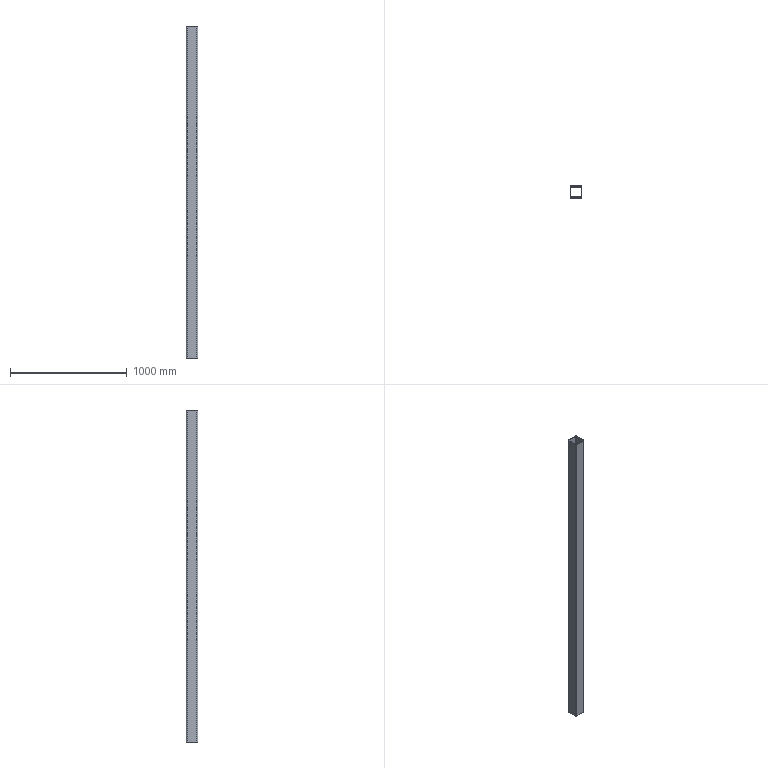Part | SolidWorks | features Extrusion 1 | 1 solid | 18 faces | box 100 x 100 x 2840 mm | volume 5213159 mm3 | plane 10 | cylinder 8 | commonest cylinder face diameters 10 x4 20 x4
STEP:
#1=CARTESIAN_POINT('',(90.,0.,2840.));
#2=VERTEX_POINT('',#1);
#3=CARTESIAN_POINT('',(100.,10.,2840.));
#4=VERTEX_POINT('',#3);
#5=CARTESIAN_POINT('',(90.,10.,2840.));
#6=DIRECTION('',(0.,0.,1.));
#7=DIRECTION('',(-1.,0.,0.));
#8=AXIS2_PLACEMENT_3D('',#5,#6,#7);
#9=CIRCLE('',#8,10.);
#10=EDGE_CURVE('',#2,#4,#9,.T.);
#11=ORIENTED_EDGE('',*,*,#10,.T.);
#12=CARTESIAN_POINT('',(100.,90.,2840.));
#13=VERTEX_POINT('',#12);
#14=CARTESIAN_POINT('',(100.,10.,2840.));
#15=DIRECTION('',(0.,1.,0.));
#16=VECTOR('',#15,1000.);
#17=LINE('',#14,#16);
#18=EDGE_CURVE('',#4,#13,#17,.T.);
#19=ORIENTED_EDGE('',*,*,#18,.T.);
#20=CARTESIAN_POINT('',(90.,100.,2840.));
#21=VERTEX_POINT('',#20);
#22=CARTESIAN_POINT('',(90.,90.,2840.));
#23=DIRECTION('',(0.,0.,1.));
#24=DIRECTION('',(1.,0.,0.));
#25=AXIS2_PLACEMENT_3D('',#22,#23,#24);
#26=CIRCLE('',#25,10.);
#27=EDGE_CURVE('',#13,#21,#26,.T.);
#28=ORIENTED_EDGE('',*,*,#27,.T.);
#29=CARTESIAN_POINT('',(10.,100.,2840.));
#30=VERTEX_POINT('',#29);
#31=CARTESIAN_POINT('',(10.,100.,2840.));
#32=DIRECTION('',(-1.,0.,0.));
#33=VECTOR('',#32,1000.);
#34=LINE('',#31,#33);
#35=EDGE_CURVE('',#21,#30,#34,.T.);
#36=ORIENTED_EDGE('',*,*,#35,.T.);
#37=CARTESIAN_POINT('',(0.,90.,2840.));
#38=VERTEX_POINT('',#37);
#39=CARTESIAN_POINT('',(10.,90.,2840.));
#40=DIRECTION('',(0.,0.,1.));
#41=DIRECTION('',(-1.,0.,0.));
#42=AXIS2_PLACEMENT_3D('',#39,#40,#41);
#43=CIRCLE('',#42,10.);
#44=EDGE_CURVE('',#30,#38,#43,.T.);
#45=ORIENTED_EDGE('',*,*,#44,.T.);
#46=CARTESIAN_POINT('',(0.,10.,2840.));
#47=VERTEX_POINT('',#46);
#48=CARTESIAN_POINT('',(0.,10.,2840.));
#49=DIRECTION('',(0.,-1.,0.));
#50=VECTOR('',#49,1000.);
#51=LINE('',#48,#50);
#52=EDGE_CURVE('',#38,#47,#51,.T.);
#53=ORIENTED_EDGE('',*,*,#52,.T.);
#54=CARTESIAN_POINT('',(10.,0.,2840.));
#55=VERTEX_POINT('',#54);
#56=CARTESIAN_POINT('',(10.,10.,2840.));
#57=DIRECTION('',(0.,0.,1.));
#58=DIRECTION('',(-1.,0.,0.));
#59=AXIS2_PLACEMENT_3D('',#56,#57,#58);
#60=CIRCLE('',#59,10.);
#61=EDGE_CURVE('',#47,#55,#60,.T.);
#62=ORIENTED_EDGE('',*,*,#61,.T.);
#63=CARTESIAN_POINT('',(10.,0.,2840.));
#64=DIRECTION('',(1.,0.,0.));
#65=VECTOR('',#64,1000.);
#66=LINE('',#63,#65);
#67=EDGE_CURVE('',#55,#2,#66,.T.);
#68=ORIENTED_EDGE('',*,*,#67,.T.);
#69=EDGE_LOOP('',(#11,#19,#28,#36,#45,#53,#62,#68));
#70=FACE_OUTER_BOUND('',#69,.T.);
#71=CARTESIAN_POINT('',(10.,95.,2840.));
#72=VERTEX_POINT('',#71);
#73=CARTESIAN_POINT('',(5.,90.,2840.));
#74=VERTEX_POINT('',#73);
#75=CARTESIAN_POINT('',(10.,90.,2840.));
#76=DIRECTION('',(0.,0.,1.));
#77=DIRECTION('',(-1.,0.,0.));
#78=AXIS2_PLACEMENT_3D('',#75,#76,#77);
#79=CIRCLE('',#78,5.);
#80=EDGE_CURVE('',#72,#74,#79,.T.);
#81=ORIENTED_EDGE('',*,*,#80,.F.);
#82=CARTESIAN_POINT('',(90.,95.,2840.));
#83=VERTEX_POINT('',#82);
#84=CARTESIAN_POINT('',(10.,95.,2840.));
#85=DIRECTION('',(-1.,0.,0.));
#86=VECTOR('',#85,1000.);
#87=LINE('',#84,#86);
#88=EDGE_CURVE('',#83,#72,#87,.T.);
#89=ORIENTED_EDGE('',*,*,#88,.F.);
#90=CARTESIAN_POINT('',(95.,90.,2840.));
#91=VERTEX_POINT('',#90);
#92=CARTESIAN_POINT('',(90.,90.,2840.));
#93=DIRECTION('',(0.,0.,1.));
#94=DIRECTION('',(1.,0.,0.));
#95=AXIS2_PLACEMENT_3D('',#92,#93,#94);
#96=CIRCLE('',#95,5.);
#97=EDGE_CURVE('',#91,#83,#96,.T.);
#98=ORIENTED_EDGE('',*,*,#97,.F.);
#99=CARTESIAN_POINT('',(95.,10.,2840.));
#100=VERTEX_POINT('',#99);
#101=CARTESIAN_POINT('',(95.,10.,2840.));
#102=DIRECTION('',(0.,1.,0.));
#103=VECTOR('',#102,1000.);
#104=LINE('',#101,#103);
#105=EDGE_CURVE('',#100,#91,#104,.T.);
#106=ORIENTED_EDGE('',*,*,#105,.F.);
#107=CARTESIAN_POINT('',(90.,5.,2840.));
#108=VERTEX_POINT('',#107);
#109=CARTESIAN_POINT('',(90.,10.,2840.));
#110=DIRECTION('',(0.,0.,1.));
#111=DIRECTION('',(-1.,0.,0.));
#112=AXIS2_PLACEMENT_3D('',#109,#110,#111);
#113=CIRCLE('',#112,5.);
#114=EDGE_CURVE('',#108,#100,#113,.T.);
#115=ORIENTED_EDGE('',*,*,#114,.F.);
#116=CARTESIAN_POINT('',(10.,5.,2840.));
#117=VERTEX_POINT('',#116);
#118=CARTESIAN_POINT('',(10.,5.,2840.));
#119=DIRECTION('',(1.,0.,0.));
#120=VECTOR('',#119,1000.);
#121=LINE('',#118,#120);
#122=EDGE_CURVE('',#117,#108,#121,.T.);
#123=ORIENTED_EDGE('',*,*,#122,.F.);
#124=CARTESIAN_POINT('',(5.,10.,2840.));
#125=VERTEX_POINT('',#124);
#126=CARTESIAN_POINT('',(10.,10.,2840.));
#127=DIRECTION('',(0.,0.,1.));
#128=DIRECTION('',(-1.,0.,0.));
#129=AXIS2_PLACEMENT_3D('',#126,#127,#128);
#130=CIRCLE('',#129,5.);
#131=EDGE_CURVE('',#125,#117,#130,.T.);
#132=ORIENTED_EDGE('',*,*,#131,.F.);
#133=CARTESIAN_POINT('',(5.,10.,2840.));
#134=DIRECTION('',(0.,-1.,0.));
#135=VECTOR('',#134,1000.);
#136=LINE('',#133,#135);
#137=EDGE_CURVE('',#74,#125,#136,.T.);
#138=ORIENTED_EDGE('',*,*,#137,.F.);
#139=EDGE_LOOP('',(#81,#89,#98,#106,#115,#123,#132,#138));
#140=FACE_BOUND('',#139,.T.);
#141=CARTESIAN_POINT('',(90.,10.,2840.));
#142=DIRECTION('',(0.,0.,-1.));
#143=DIRECTION('',(-1.,0.,0.));
#144=AXIS2_PLACEMENT_3D('',#141,#142,#143);
#145=PLANE('',#144);
#146=ADVANCED_FACE('',(#70,#140),#145,.F.);
#147=CARTESIAN_POINT('',(90.,0.,0.));
#148=VERTEX_POINT('',#147);
#149=CARTESIAN_POINT('',(100.,10.,0.));
#150=VERTEX_POINT('',#149);
#151=CARTESIAN_POINT('',(90.,10.,0.));
#152=DIRECTION('',(0.,0.,1.));
#153=DIRECTION('',(-1.,0.,0.));
#154=AXIS2_PLACEMENT_3D('',#151,#152,#153);
#155=CIRCLE('',#154,10.);
#156=EDGE_CURVE('',#148,#150,#155,.T.);
#157=ORIENTED_EDGE('',*,*,#156,.F.);
#158=CARTESIAN_POINT('',(10.,0.,0.));
#159=VERTEX_POINT('',#158);
#160=CARTESIAN_POINT('',(10.,0.,0.));
#161=DIRECTION('',(1.,0.,0.));
#162=VECTOR('',#161,1000.);
#163=LINE('',#160,#162);
#164=EDGE_CURVE('',#159,#148,#163,.T.);
#165=ORIENTED_EDGE('',*,*,#164,.F.);
#166=CARTESIAN_POINT('',(0.,10.,0.));
#167=VERTEX_POINT('',#166);
#168=CARTESIAN_POINT('',(10.,10.,0.));
#169=DIRECTION('',(0.,0.,1.));
#170=DIRECTION('',(-1.,0.,0.));
#171=AXIS2_PLACEMENT_3D('',#168,#169,#170);
#172=CIRCLE('',#171,10.);
#173=EDGE_CURVE('',#167,#159,#172,.T.);
#174=ORIENTED_EDGE('',*,*,#173,.F.);
#175=CARTESIAN_POINT('',(0.,90.,0.));
#176=VERTEX_POINT('',#175);
#177=CARTESIAN_POINT('',(0.,10.,0.));
#178=DIRECTION('',(0.,-1.,0.));
#179=VECTOR('',#178,1000.);
#180=LINE('',#177,#179);
#181=EDGE_CURVE('',#176,#167,#180,.T.);
#182=ORIENTED_EDGE('',*,*,#181,.F.);
#183=CARTESIAN_POINT('',(10.,100.,0.));
#184=VERTEX_POINT('',#183);
#185=CARTESIAN_POINT('',(10.,90.,0.));
#186=DIRECTION('',(0.,0.,1.));
#187=DIRECTION('',(-1.,0.,0.));
#188=AXIS2_PLACEMENT_3D('',#185,#186,#187);
#189=CIRCLE('',#188,10.);
#190=EDGE_CURVE('',#184,#176,#189,.T.);
#191=ORIENTED_EDGE('',*,*,#190,.F.);
#192=CARTESIAN_POINT('',(90.,100.,0.));
#193=VERTEX_POINT('',#192);
#194=CARTESIAN_POINT('',(10.,100.,0.));
#195=DIRECTION('',(-1.,0.,0.));
#196=VECTOR('',#195,1000.);
#197=LINE('',#194,#196);
#198=EDGE_CURVE('',#193,#184,#197,.T.);
#199=ORIENTED_EDGE('',*,*,#198,.F.);
#200=CARTESIAN_POINT('',(100.,90.,0.));
#201=VERTEX_POINT('',#200);
#202=CARTESIAN_POINT('',(90.,90.,0.));
#203=DIRECTION('',(0.,0.,1.));
#204=DIRECTION('',(1.,0.,0.));
#205=AXIS2_PLACEMENT_3D('',#202,#203,#204);
#206=CIRCLE('',#205,10.);
#207=EDGE_CURVE('',#201,#193,#206,.T.);
#208=ORIENTED_EDGE('',*,*,#207,.F.);
#209=CARTESIAN_POINT('',(100.,10.,0.));
#210=DIRECTION('',(0.,1.,0.));
#211=VECTOR('',#210,1000.);
#212=LINE('',#209,#211);
#213=EDGE_CURVE('',#150,#201,#212,.T.);
#214=ORIENTED_EDGE('',*,*,#213,.F.);
#215=EDGE_LOOP('',(#157,#165,#174,#182,#191,#199,#208,#214));
#216=FACE_OUTER_BOUND('',#215,.T.);
#217=CARTESIAN_POINT('',(90.,95.,0.));
#218=VERTEX_POINT('',#217);
#219=CARTESIAN_POINT('',(10.,95.,0.));
#220=VERTEX_POINT('',#219);
#221=CARTESIAN_POINT('',(10.,95.,0.));
#222=DIRECTION('',(-1.,0.,0.));
#223=VECTOR('',#222,1000.);
#224=LINE('',#221,#223);
#225=EDGE_CURVE('',#218,#220,#224,.T.);
#226=ORIENTED_EDGE('',*,*,#225,.T.);
#227=CARTESIAN_POINT('',(5.,90.,0.));
#228=VERTEX_POINT('',#227);
#229=CARTESIAN_POINT('',(10.,90.,0.));
#230=DIRECTION('',(0.,0.,1.));
#231=DIRECTION('',(-1.,0.,0.));
#232=AXIS2_PLACEMENT_3D('',#229,#230,#231);
#233=CIRCLE('',#232,5.);
#234=EDGE_CURVE('',#220,#228,#233,.T.);
#235=ORIENTED_EDGE('',*,*,#234,.T.);
#236=CARTESIAN_POINT('',(5.,10.,0.));
#237=VERTEX_POINT('',#236);
#238=CARTESIAN_POINT('',(5.,10.,0.));
#239=DIRECTION('',(0.,-1.,0.));
#240=VECTOR('',#239,1000.);
#241=LINE('',#238,#240);
#242=EDGE_CURVE('',#228,#237,#241,.T.);
#243=ORIENTED_EDGE('',*,*,#242,.T.);
#244=CARTESIAN_POINT('',(10.,5.,0.));
#245=VERTEX_POINT('',#244);
#246=CARTESIAN_POINT('',(10.,10.,0.));
#247=DIRECTION('',(0.,0.,1.));
#248=DIRECTION('',(-1.,0.,0.));
#249=AXIS2_PLACEMENT_3D('',#246,#247,#248);
#250=CIRCLE('',#249,5.);
#251=EDGE_CURVE('',#237,#245,#250,.T.);
#252=ORIENTED_EDGE('',*,*,#251,.T.);
#253=CARTESIAN_POINT('',(90.,5.,0.));
#254=VERTEX_POINT('',#253);
#255=CARTESIAN_POINT('',(10.,5.,0.));
#256=DIRECTION('',(1.,0.,0.));
#257=VECTOR('',#256,1000.);
#258=LINE('',#255,#257);
#259=EDGE_CURVE('',#245,#254,#258,.T.);
#260=ORIENTED_EDGE('',*,*,#259,.T.);
#261=CARTESIAN_POINT('',(95.,10.,0.));
#262=VERTEX_POINT('',#261);
#263=CARTESIAN_POINT('',(90.,10.,0.));
#264=DIRECTION('',(0.,0.,1.));
#265=DIRECTION('',(-1.,0.,0.));
#266=AXIS2_PLACEMENT_3D('',#263,#264,#265);
#267=CIRCLE('',#266,5.);
#268=EDGE_CURVE('',#254,#262,#267,.T.);
#269=ORIENTED_EDGE('',*,*,#268,.T.);
#270=CARTESIAN_POINT('',(95.,90.,0.));
#271=VERTEX_POINT('',#270);
#272=CARTESIAN_POINT('',(95.,10.,0.));
#273=DIRECTION('',(0.,1.,0.));
#274=VECTOR('',#273,1000.);
#275=LINE('',#272,#274);
#276=EDGE_CURVE('',#262,#271,#275,.T.);
#277=ORIENTED_EDGE('',*,*,#276,.T.);
#278=CARTESIAN_POINT('',(90.,90.,0.));
#279=DIRECTION('',(0.,0.,1.));
#280=DIRECTION('',(1.,0.,0.));
#281=AXIS2_PLACEMENT_3D('',#278,#279,#280);
#282=CIRCLE('',#281,5.);
#283=EDGE_CURVE('',#271,#218,#282,.T.);
#284=ORIENTED_EDGE('',*,*,#283,.T.);
#285=EDGE_LOOP('',(#226,#235,#243,#252,#260,#269,#277,#284));
#286=FACE_BOUND('',#285,.T.);
#287=CARTESIAN_POINT('',(90.,10.,0.));
#288=DIRECTION('',(0.,0.,-1.));
#289=DIRECTION('',(-1.,0.,0.));
#290=AXIS2_PLACEMENT_3D('',#287,#288,#289);
#291=PLANE('',#290);
#292=ADVANCED_FACE('',(#216,#286),#291,.T.);
#293=ORIENTED_EDGE('',*,*,#156,.T.);
#294=CARTESIAN_POINT('',(100.,10.,2840.));
#295=DIRECTION('',(0.,0.,-1.));
#296=VECTOR('',#295,1000.);
#297=LINE('',#294,#296);
#298=EDGE_CURVE('',#4,#150,#297,.T.);
#299=ORIENTED_EDGE('',*,*,#298,.F.);
#300=ORIENTED_EDGE('',*,*,#10,.F.);
#301=CARTESIAN_POINT('',(90.,0.,2840.));
#302=DIRECTION('',(0.,0.,-1.));
#303=VECTOR('',#302,1000.);
#304=LINE('',#301,#303);
#305=EDGE_CURVE('',#2,#148,#304,.T.);
#306=ORIENTED_EDGE('',*,*,#305,.T.);
#307=EDGE_LOOP('',(#293,#299,#300,#306));
#308=FACE_OUTER_BOUND('',#307,.T.);
#309=CARTESIAN_POINT('',(90.,10.,2840.));
#310=DIRECTION('',(0.,0.,-1.));
#311=DIRECTION('',(-1.,0.,0.));
#312=AXIS2_PLACEMENT_3D('',#309,#310,#311);
#313=CYLINDRICAL_SURFACE('',#312,10.);
#314=ADVANCED_FACE('',(#308),#313,.T.);
#315=ORIENTED_EDGE('',*,*,#213,.T.);
#316=CARTESIAN_POINT('',(100.,90.,2840.));
#317=DIRECTION('',(0.,0.,-1.));
#318=VECTOR('',#317,1000.);
#319=LINE('',#316,#318);
#320=EDGE_CURVE('',#13,#201,#319,.T.);
#321=ORIENTED_EDGE('',*,*,#320,.F.);
#322=ORIENTED_EDGE('',*,*,#18,.F.);
#323=ORIENTED_EDGE('',*,*,#298,.T.);
#324=EDGE_LOOP('',(#315,#321,#322,#323));
#325=FACE_OUTER_BOUND('',#324,.T.);
#326=CARTESIAN_POINT('',(100.,10.,2840.));
#327=DIRECTION('',(-1.,0.,0.));
#328=DIRECTION('',(0.,-1.,0.));
#329=AXIS2_PLACEMENT_3D('',#326,#327,#328);
#330=PLANE('',#329);
#331=ADVANCED_FACE('',(#325),#330,.F.);
#332=ORIENTED_EDGE('',*,*,#207,.T.);
#333=CARTESIAN_POINT('',(90.,100.,2840.));
#334=DIRECTION('',(0.,0.,-1.));
#335=VECTOR('',#334,1000.);
#336=LINE('',#333,#335);
#337=EDGE_CURVE('',#21,#193,#336,.T.);
#338=ORIENTED_EDGE('',*,*,#337,.F.);
#339=ORIENTED_EDGE('',*,*,#27,.F.);
#340=ORIENTED_EDGE('',*,*,#320,.T.);
#341=EDGE_LOOP('',(#332,#338,#339,#340));
#342=FACE_OUTER_BOUND('',#341,.T.);
#343=CARTESIAN_POINT('',(90.,90.,2840.));
#344=DIRECTION('',(0.,0.,-1.));
#345=DIRECTION('',(-1.,0.,0.));
#346=AXIS2_PLACEMENT_3D('',#343,#344,#345);
#347=CYLINDRICAL_SURFACE('',#346,10.);
#348=ADVANCED_FACE('',(#342),#347,.T.);
#349=ORIENTED_EDGE('',*,*,#198,.T.);
#350=CARTESIAN_POINT('',(10.,100.,2840.));
#351=DIRECTION('',(0.,0.,-1.));
#352=VECTOR('',#351,1000.);
#353=LINE('',#350,#352);
#354=EDGE_CURVE('',#30,#184,#353,.T.);
#355=ORIENTED_EDGE('',*,*,#354,.F.);
#356=ORIENTED_EDGE('',*,*,#35,.F.);
#357=ORIENTED_EDGE('',*,*,#337,.T.);
#358=EDGE_LOOP('',(#349,#355,#356,#357));
#359=FACE_OUTER_BOUND('',#358,.T.);
#360=CARTESIAN_POINT('',(10.,100.,2840.));
#361=DIRECTION('',(0.,-1.,0.));
#362=DIRECTION('',(0.,0.,-1.));
#363=AXIS2_PLACEMENT_3D('',#360,#361,#362);
#364=PLANE('',#363);
#365=ADVANCED_FACE('',(#359),#364,.F.);
#366=ORIENTED_EDGE('',*,*,#190,.T.);
#367=CARTESIAN_POINT('',(0.,90.,2840.));
#368=DIRECTION('',(0.,0.,-1.));
#369=VECTOR('',#368,1000.);
#370=LINE('',#367,#369);
#371=EDGE_CURVE('',#38,#176,#370,.T.);
#372=ORIENTED_EDGE('',*,*,#371,.F.);
#373=ORIENTED_EDGE('',*,*,#44,.F.);
#374=ORIENTED_EDGE('',*,*,#354,.T.);
#375=EDGE_LOOP('',(#366,#372,#373,#374));
#376=FACE_OUTER_BOUND('',#375,.T.);
#377=CARTESIAN_POINT('',(10.,90.,2840.));
#378=DIRECTION('',(0.,0.,-1.));
#379=DIRECTION('',(-1.,0.,0.));
#380=AXIS2_PLACEMENT_3D('',#377,#378,#379);
#381=CYLINDRICAL_SURFACE('',#380,10.);
#382=ADVANCED_FACE('',(#376),#381,.T.);
#383=ORIENTED_EDGE('',*,*,#181,.T.);
#384=CARTESIAN_POINT('',(0.,10.,2840.));
#385=DIRECTION('',(0.,0.,-1.));
#386=VECTOR('',#385,1000.);
#387=LINE('',#384,#386);
#388=EDGE_CURVE('',#47,#167,#387,.T.);
#389=ORIENTED_EDGE('',*,*,#388,.F.);
#390=ORIENTED_EDGE('',*,*,#52,.F.);
#391=ORIENTED_EDGE('',*,*,#371,.T.);
#392=EDGE_LOOP('',(#383,#389,#390,#391));
#393=FACE_OUTER_BOUND('',#392,.T.);
#394=CARTESIAN_POINT('',(0.,10.,2840.));
#395=DIRECTION('',(1.,0.,0.));
#396=DIRECTION('',(0.,1.,0.));
#397=AXIS2_PLACEMENT_3D('',#394,#395,#396);
#398=PLANE('',#397);
#399=ADVANCED_FACE('',(#393),#398,.F.);
#400=ORIENTED_EDGE('',*,*,#173,.T.);
#401=CARTESIAN_POINT('',(10.,0.,2840.));
#402=DIRECTION('',(0.,0.,-1.));
#403=VECTOR('',#402,1000.);
#404=LINE('',#401,#403);
#405=EDGE_CURVE('',#55,#159,#404,.T.);
#406=ORIENTED_EDGE('',*,*,#405,.F.);
#407=ORIENTED_EDGE('',*,*,#61,.F.);
#408=ORIENTED_EDGE('',*,*,#388,.T.);
#409=EDGE_LOOP('',(#400,#406,#407,#408));
#410=FACE_OUTER_BOUND('',#409,.T.);
#411=CARTESIAN_POINT('',(10.,10.,2840.));
#412=DIRECTION('',(0.,0.,-1.));
#413=DIRECTION('',(-1.,0.,0.));
#414=AXIS2_PLACEMENT_3D('',#411,#412,#413);
#415=CYLINDRICAL_SURFACE('',#414,10.);
#416=ADVANCED_FACE('',(#410),#415,.T.);
#417=ORIENTED_EDGE('',*,*,#164,.T.);
#418=ORIENTED_EDGE('',*,*,#305,.F.);
#419=ORIENTED_EDGE('',*,*,#67,.F.);
#420=ORIENTED_EDGE('',*,*,#405,.T.);
#421=EDGE_LOOP('',(#417,#418,#419,#420));
#422=FACE_OUTER_BOUND('',#421,.T.);
#423=CARTESIAN_POINT('',(10.,0.,2840.));
#424=DIRECTION('',(0.,1.,0.));
#425=DIRECTION('',(0.,0.,1.));
#426=AXIS2_PLACEMENT_3D('',#423,#424,#425);
#427=PLANE('',#426);
#428=ADVANCED_FACE('',(#422),#427,.F.);
#429=ORIENTED_EDGE('',*,*,#234,.F.);
#430=CARTESIAN_POINT('',(10.,95.,2840.));
#431=DIRECTION('',(0.,0.,-1.));
#432=VECTOR('',#431,1000.);
#433=LINE('',#430,#432);
#434=EDGE_CURVE('',#72,#220,#433,.T.);
#435=ORIENTED_EDGE('',*,*,#434,.F.);
#436=ORIENTED_EDGE('',*,*,#80,.T.);
#437=CARTESIAN_POINT('',(5.,90.,2840.));
#438=DIRECTION('',(0.,0.,-1.));
#439=VECTOR('',#438,1000.);
#440=LINE('',#437,#439);
#441=EDGE_CURVE('',#74,#228,#440,.T.);
#442=ORIENTED_EDGE('',*,*,#441,.T.);
#443=EDGE_LOOP('',(#429,#435,#436,#442));
#444=FACE_OUTER_BOUND('',#443,.T.);
#445=CARTESIAN_POINT('',(10.,90.,2840.));
#446=DIRECTION('',(0.,0.,-1.));
#447=DIRECTION('',(-1.,0.,0.));
#448=AXIS2_PLACEMENT_3D('',#445,#446,#447);
#449=CYLINDRICAL_SURFACE('',#448,5.);
#450=ADVANCED_FACE('',(#444),#449,.F.);
#451=ORIENTED_EDGE('',*,*,#242,.F.);
#452=ORIENTED_EDGE('',*,*,#441,.F.);
#453=ORIENTED_EDGE('',*,*,#137,.T.);
#454=CARTESIAN_POINT('',(5.,10.,2840.));
#455=DIRECTION('',(0.,0.,-1.));
#456=VECTOR('',#455,1000.);
#457=LINE('',#454,#456);
#458=EDGE_CURVE('',#125,#237,#457,.T.);
#459=ORIENTED_EDGE('',*,*,#458,.T.);
#460=EDGE_LOOP('',(#451,#452,#453,#459));
#461=FACE_OUTER_BOUND('',#460,.T.);
#462=CARTESIAN_POINT('',(5.,10.,2840.));
#463=DIRECTION('',(1.,0.,0.));
#464=DIRECTION('',(0.,1.,0.));
#465=AXIS2_PLACEMENT_3D('',#462,#463,#464);
#466=PLANE('',#465);
#467=ADVANCED_FACE('',(#461),#466,.T.);
#468=ORIENTED_EDGE('',*,*,#251,.F.);
#469=ORIENTED_EDGE('',*,*,#458,.F.);
#470=ORIENTED_EDGE('',*,*,#131,.T.);
#471=CARTESIAN_POINT('',(10.,5.,2840.));
#472=DIRECTION('',(0.,0.,-1.));
#473=VECTOR('',#472,1000.);
#474=LINE('',#471,#473);
#475=EDGE_CURVE('',#117,#245,#474,.T.);
#476=ORIENTED_EDGE('',*,*,#475,.T.);
#477=EDGE_LOOP('',(#468,#469,#470,#476));
#478=FACE_OUTER_BOUND('',#477,.T.);
#479=CARTESIAN_POINT('',(10.,10.,2840.));
#480=DIRECTION('',(0.,0.,-1.));
#481=DIRECTION('',(-1.,0.,0.));
#482=AXIS2_PLACEMENT_3D('',#479,#480,#481);
#483=CYLINDRICAL_SURFACE('',#482,5.);
#484=ADVANCED_FACE('',(#478),#483,.F.);
#485=ORIENTED_EDGE('',*,*,#259,.F.);
#486=ORIENTED_EDGE('',*,*,#475,.F.);
#487=ORIENTED_EDGE('',*,*,#122,.T.);
#488=CARTESIAN_POINT('',(90.,5.,2840.));
#489=DIRECTION('',(0.,0.,-1.));
#490=VECTOR('',#489,1000.);
#491=LINE('',#488,#490);
#492=EDGE_CURVE('',#108,#254,#491,.T.);
#493=ORIENTED_EDGE('',*,*,#492,.T.);
#494=EDGE_LOOP('',(#485,#486,#487,#493));
#495=FACE_OUTER_BOUND('',#494,.T.);
#496=CARTESIAN_POINT('',(10.,5.,2840.));
#497=DIRECTION('',(0.,1.,0.));
#498=DIRECTION('',(0.,0.,1.));
#499=AXIS2_PLACEMENT_3D('',#496,#497,#498);
#500=PLANE('',#499);
#501=ADVANCED_FACE('',(#495),#500,.T.);
#502=ORIENTED_EDGE('',*,*,#268,.F.);
#503=ORIENTED_EDGE('',*,*,#492,.F.);
#504=ORIENTED_EDGE('',*,*,#114,.T.);
#505=CARTESIAN_POINT('',(95.,10.,2840.));
#506=DIRECTION('',(0.,0.,-1.));
#507=VECTOR('',#506,1000.);
#508=LINE('',#505,#507);
#509=EDGE_CURVE('',#100,#262,#508,.T.);
#510=ORIENTED_EDGE('',*,*,#509,.T.);
#511=EDGE_LOOP('',(#502,#503,#504,#510));
#512=FACE_OUTER_BOUND('',#511,.T.);
#513=CARTESIAN_POINT('',(90.,10.,2840.));
#514=DIRECTION('',(0.,0.,-1.));
#515=DIRECTION('',(-1.,0.,0.));
#516=AXIS2_PLACEMENT_3D('',#513,#514,#515);
#517=CYLINDRICAL_SURFACE('',#516,5.);
#518=ADVANCED_FACE('',(#512),#517,.F.);
#519=ORIENTED_EDGE('',*,*,#276,.F.);
#520=ORIENTED_EDGE('',*,*,#509,.F.);
#521=ORIENTED_EDGE('',*,*,#105,.T.);
#522=CARTESIAN_POINT('',(95.,90.,2840.));
#523=DIRECTION('',(0.,0.,-1.));
#524=VECTOR('',#523,1000.);
#525=LINE('',#522,#524);
#526=EDGE_CURVE('',#91,#271,#525,.T.);
#527=ORIENTED_EDGE('',*,*,#526,.T.);
#528=EDGE_LOOP('',(#519,#520,#521,#527));
#529=FACE_OUTER_BOUND('',#528,.T.);
#530=CARTESIAN_POINT('',(95.,10.,2840.));
#531=DIRECTION('',(-1.,0.,0.));
#532=DIRECTION('',(0.,-1.,0.));
#533=AXIS2_PLACEMENT_3D('',#530,#531,#532);
#534=PLANE('',#533);
#535=ADVANCED_FACE('',(#529),#534,.T.);
#536=ORIENTED_EDGE('',*,*,#283,.F.);
#537=ORIENTED_EDGE('',*,*,#526,.F.);
#538=ORIENTED_EDGE('',*,*,#97,.T.);
#539=CARTESIAN_POINT('',(90.,95.,2840.));
#540=DIRECTION('',(0.,0.,-1.));
#541=VECTOR('',#540,1000.);
#542=LINE('',#539,#541);
#543=EDGE_CURVE('',#83,#218,#542,.T.);
#544=ORIENTED_EDGE('',*,*,#543,.T.);
#545=EDGE_LOOP('',(#536,#537,#538,#544));
#546=FACE_OUTER_BOUND('',#545,.T.);
#547=CARTESIAN_POINT('',(90.,90.,2840.));
#548=DIRECTION('',(0.,0.,-1.));
#549=DIRECTION('',(-1.,0.,0.));
#550=AXIS2_PLACEMENT_3D('',#547,#548,#549);
#551=CYLINDRICAL_SURFACE('',#550,5.);
#552=ADVANCED_FACE('',(#546),#551,.F.);
#553=ORIENTED_EDGE('',*,*,#225,.F.);
#554=ORIENTED_EDGE('',*,*,#543,.F.);
#555=ORIENTED_EDGE('',*,*,#88,.T.);
#556=ORIENTED_EDGE('',*,*,#434,.T.);
#557=EDGE_LOOP('',(#553,#554,#555,#556));
#558=FACE_OUTER_BOUND('',#557,.T.);
#559=CARTESIAN_POINT('',(10.,95.,2840.));
#560=DIRECTION('',(0.,-1.,0.));
#561=DIRECTION('',(0.,0.,-1.));
#562=AXIS2_PLACEMENT_3D('',#559,#560,#561);
#563=PLANE('',#562);
#564=ADVANCED_FACE('',(#558),#563,.T.);
#565=CLOSED_SHELL('',(#146,#292,#314,#331,#348,#365,#382,#399,#416,#428,#450,#467,#484,#501,#518,#535,#552,#564));
#566=MANIFOLD_SOLID_BREP('',#565);
#567=CARTESIAN_POINT('',(0.,0.,0.));
#568=DIRECTION('',(0.,0.,1.));
#569=DIRECTION('',(1.,0.,0.));
#570=AXIS2_PLACEMENT_3D('',#567,#568,#569);
#571=(LENGTH_UNIT()NAMED_UNIT(*)SI_UNIT(.MILLI.,.METRE.));
#572=UNCERTAINTY_MEASURE_WITH_UNIT(LENGTH_MEASURE(0.00001),#571,'','');
#573=(NAMED_UNIT(*)PLANE_ANGLE_UNIT()SI_UNIT($,.RADIAN.));
#574=(NAMED_UNIT(*)SI_UNIT($,.STERADIAN.)SOLID_ANGLE_UNIT());
#575=(GEOMETRIC_REPRESENTATION_CONTEXT(3)GLOBAL_UNCERTAINTY_ASSIGNED_CONTEXT((#572))GLOBAL_UNIT_ASSIGNED_CONTEXT((#571,#573,#574))REPRESENTATION_CONTEXT('',''));
#576=ADVANCED_BREP_SHAPE_REPRESENTATION('',(#566,#570),#575);